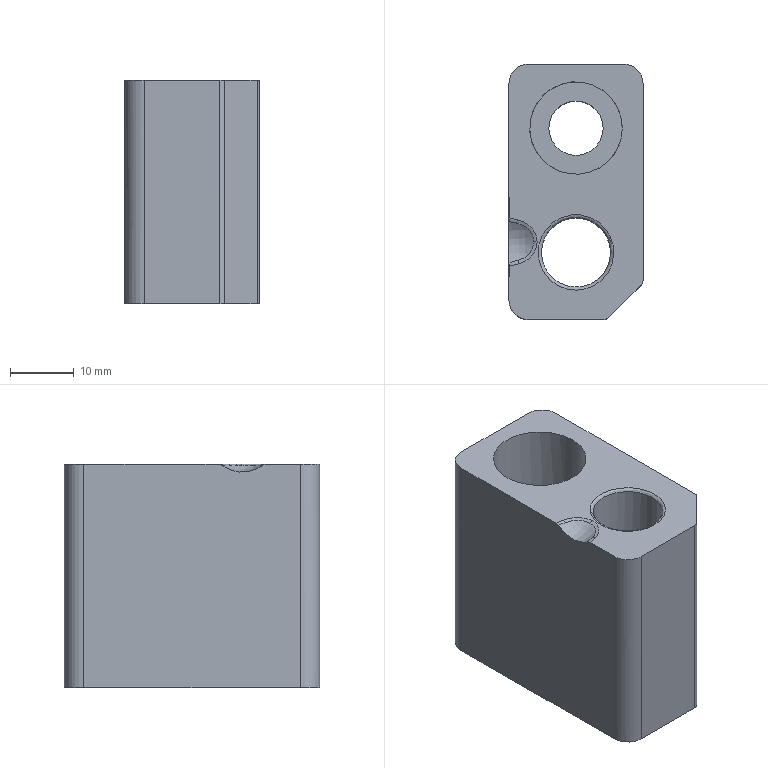Part | NX | features DIE-21 2 | 1 solid | 24 faces | box 21.001 x 40 x 35 mm | volume 21730 mm3 | plane 9 | cylinder 9 | spline 5 | torus 1 | commonest cylinder face diameters 6 x3 2 x2 8.506 x1 10.85 x1 14.5 x1 15 x1
STEP:
#1=CARTESIAN_POINT('',(2448.597,-804.612,858.547));
#2=VERTEX_POINT('',#1);
#3=CARTESIAN_POINT('',(2448.597,-811.041,858.549));
#4=VERTEX_POINT('',#3);
#5=CARTESIAN_POINT('',(2448.597,-804.616,858.545));
#6=CARTESIAN_POINT('',(2448.597,-805.575,857.92));
#7=CARTESIAN_POINT('',(2448.597,-807.823,857.052));
#8=CARTESIAN_POINT('',(2448.597,-810.077,857.926));
#9=CARTESIAN_POINT('',(2448.597,-811.039,858.548));
#10=B_SPLINE_CURVE_WITH_KNOTS('',3,(#5,#6,#7,#8,#9),.UNSPECIFIED.,.F.,.F.,(4,1,4),(0.0003039,0.003718,0.007132),.UNSPECIFIED.);
#11=EDGE_CURVE('',#2,#4,#10,.T.);
#12=ORIENTED_EDGE('',*,*,#11,.F.);
#13=CARTESIAN_POINT('',(2448.599,-804.048,858.716));
#14=VERTEX_POINT('',#13);
#15=CARTESIAN_POINT('',(2448.597,-804.617,858.543));
#16=CARTESIAN_POINT('',(2448.597,-804.449,858.653));
#17=CARTESIAN_POINT('',(2448.597,-804.249,858.716));
#18=CARTESIAN_POINT('',(2448.597,-804.048,858.716));
#19=B_SPLINE_CURVE_WITH_KNOTS('',3,(#15,#16,#17,#18),.UNSPECIFIED.,.F.,.F.,(4,4),(0.,0.0006043),.UNSPECIFIED.);
#20=EDGE_CURVE('',#2,#14,#19,.T.);
#21=ORIENTED_EDGE('',*,*,#20,.T.);
#22=CARTESIAN_POINT('',(2448.597,-792.622,858.716));
#23=VERTEX_POINT('',#22);
#24=CARTESIAN_POINT('',(2448.597,-799.949,858.716));
#25=DIRECTION('',(0.,1.,0.));
#26=VECTOR('',#25,1000.);
#27=LINE('',#24,#26);
#28=EDGE_CURVE('',#14,#23,#27,.T.);
#29=ORIENTED_EDGE('',*,*,#28,.T.);
#30=CARTESIAN_POINT('',(2448.597,-782.949,858.716));
#31=VERTEX_POINT('',#30);
#32=CARTESIAN_POINT('',(2448.597,-792.622,858.716));
#33=CARTESIAN_POINT('',(2448.597,-789.398,858.716));
#34=CARTESIAN_POINT('',(2448.597,-786.173,858.716));
#35=CARTESIAN_POINT('',(2448.597,-782.949,858.716));
#36=B_SPLINE_CURVE_WITH_KNOTS('',3,(#32,#33,#34,#35),.UNSPECIFIED.,.F.,.F.,(4,4),(0.7155,1.),.UNSPECIFIED.);
#37=EDGE_CURVE('',#23,#31,#36,.T.);
#38=ORIENTED_EDGE('',*,*,#37,.T.);
#39=CARTESIAN_POINT('',(2448.597,-782.949,823.716));
#40=VERTEX_POINT('',#39);
#41=CARTESIAN_POINT('',(2448.597,-782.949,858.716));
#42=DIRECTION('',(0.,0.,-1.));
#43=VECTOR('',#42,1000.);
#44=LINE('',#41,#43);
#45=EDGE_CURVE('',#31,#40,#44,.T.);
#46=ORIENTED_EDGE('',*,*,#45,.T.);
#47=CARTESIAN_POINT('',(2448.597,-816.949,823.716));
#48=VERTEX_POINT('',#47);
#49=CARTESIAN_POINT('',(2448.597,-799.949,823.716));
#50=DIRECTION('',(0.,-1.,0.));
#51=VECTOR('',#50,1000.);
#52=LINE('',#49,#51);
#53=EDGE_CURVE('',#40,#48,#52,.T.);
#54=ORIENTED_EDGE('',*,*,#53,.T.);
#55=CARTESIAN_POINT('',(2448.597,-816.949,858.716));
#56=VERTEX_POINT('',#55);
#57=CARTESIAN_POINT('',(2448.597,-816.949,858.716));
#58=DIRECTION('',(0.,0.,-1.));
#59=VECTOR('',#58,1000.);
#60=LINE('',#57,#59);
#61=EDGE_CURVE('',#48,#56,#60,.F.);
#62=ORIENTED_EDGE('',*,*,#61,.T.);
#63=CARTESIAN_POINT('',(2448.599,-811.606,858.716));
#64=VERTEX_POINT('',#63);
#65=CARTESIAN_POINT('',(2448.597,-799.949,858.716));
#66=DIRECTION('',(0.,1.,0.));
#67=VECTOR('',#66,1000.);
#68=LINE('',#65,#67);
#69=EDGE_CURVE('',#56,#64,#68,.T.);
#70=ORIENTED_EDGE('',*,*,#69,.T.);
#71=CARTESIAN_POINT('',(2448.597,-811.042,858.55));
#72=CARTESIAN_POINT('',(2448.597,-811.21,858.658));
#73=CARTESIAN_POINT('',(2448.597,-811.407,858.716));
#74=CARTESIAN_POINT('',(2448.597,-811.607,858.716));
#75=B_SPLINE_CURVE_WITH_KNOTS('',3,(#71,#72,#73,#74),.UNSPECIFIED.,.F.,.F.,(4,4),(0.,0.0005946),.UNSPECIFIED.);
#76=EDGE_CURVE('',#4,#64,#75,.T.);
#77=ORIENTED_EDGE('',*,*,#76,.F.);
#78=EDGE_LOOP('',(#12,#21,#29,#38,#46,#54,#62,#70,#77));
#79=FACE_BOUND('',#78,.T.);
#80=CARTESIAN_POINT('',(2448.597,-799.949,858.716));
#81=DIRECTION('',(-1.,0.,0.));
#82=DIRECTION('',(0.,0.,1.));
#83=AXIS2_PLACEMENT_3D('',#80,#81,#82);
#84=PLANE('',#83);
#85=ADVANCED_FACE('',(#79),#84,.T.);
#86=CARTESIAN_POINT('',(2465.836,-792.622,858.716));
#87=VERTEX_POINT('',#86);
#88=CARTESIAN_POINT('',(2466.479,-787.763,858.716));
#89=CARTESIAN_POINT('',(2466.552,-791.853,858.716));
#90=CARTESIAN_POINT('',(2464.453,-795.106,858.716));
#91=CARTESIAN_POINT('',(2462.087,-796.76,858.716));
#92=CARTESIAN_POINT('',(2459.253,-797.386,858.716));
#93=CARTESIAN_POINT('',(2456.395,-796.879,858.716));
#94=CARTESIAN_POINT('',(2453.948,-795.318,858.716));
#95=CARTESIAN_POINT('',(2452.286,-792.938,858.716));
#96=CARTESIAN_POINT('',(2451.66,-790.104,858.716));
#97=CARTESIAN_POINT('',(2452.167,-787.246,858.716));
#98=CARTESIAN_POINT('',(2453.728,-784.8,858.716));
#99=CARTESIAN_POINT('',(2456.107,-783.137,858.716));
#100=CARTESIAN_POINT('',(2458.942,-782.512,858.716));
#101=CARTESIAN_POINT('',(2461.8,-783.018,858.716));
#102=CARTESIAN_POINT('',(2464.245,-784.58,858.716));
#103=CARTESIAN_POINT('',(2466.479,-787.763,858.716));
#104=CARTESIAN_POINT('',(2466.552,-791.853,858.716));
#105=CARTESIAN_POINT('',(2464.453,-795.106,858.716));
#106=B_SPLINE_CURVE_WITH_KNOTS('',3,(#88,#89,#90,#91,#92,#93,#94,#95,#96,#97,#98,#99,#100,#101,#102,#103,#104,#105),.UNSPECIFIED.,.T.,.F.,(1,1,1,1,1,1,1,1,1,1,1,1,1,1,1,1,1,1,1,1,1,1),(-0.1908,-0.1283,-0.06579,0.06013,0.1217,0.1842,0.2467,0.3092,0.3717,0.4342,0.4967,0.5592,0.6217,0.6842,0.7467,0.8092,0.8717,0.9342,1.06,1.122,1.184,1.247),.UNSPECIFIED.);
#107=EDGE_CURVE('',#87,#87,#106,.T.);
#108=ORIENTED_EDGE('',*,*,#107,.T.);
#109=EDGE_LOOP('',(#108));
#110=FACE_BOUND('',#109,.T.);
#111=CARTESIAN_POINT('',(2469.597,-792.622,858.716));
#112=VERTEX_POINT('',#111);
#113=CARTESIAN_POINT('',(2469.597,-813.827,858.716));
#114=VERTEX_POINT('',#113);
#115=CARTESIAN_POINT('',(2469.597,-799.949,858.716));
#116=DIRECTION('',(0.,1.,0.));
#117=VECTOR('',#116,1000.);
#118=LINE('',#115,#117);
#119=EDGE_CURVE('',#112,#114,#118,.F.);
#120=ORIENTED_EDGE('',*,*,#119,.F.);
#121=CARTESIAN_POINT('',(2469.597,-782.949,858.716));
#122=VERTEX_POINT('',#121);
#123=CARTESIAN_POINT('',(2469.597,-792.622,858.716));
#124=CARTESIAN_POINT('',(2469.597,-789.398,858.716));
#125=CARTESIAN_POINT('',(2469.597,-786.173,858.716));
#126=CARTESIAN_POINT('',(2469.597,-782.949,858.716));
#127=B_SPLINE_CURVE_WITH_KNOTS('',3,(#123,#124,#125,#126),.UNSPECIFIED.,.F.,.F.,(4,4),(0.6937,1.),.UNSPECIFIED.);
#128=EDGE_CURVE('',#122,#112,#127,.F.);
#129=ORIENTED_EDGE('',*,*,#128,.F.);
#130=CARTESIAN_POINT('',(2466.597,-779.949,858.716));
#131=VERTEX_POINT('',#130);
#132=CARTESIAN_POINT('',(2466.597,-782.949,858.716));
#133=DIRECTION('',(0.,0.,1.));
#134=DIRECTION('',(1.,0.,0.));
#135=AXIS2_PLACEMENT_3D('',#132,#133,#134);
#136=CIRCLE('',#135,3.);
#137=EDGE_CURVE('',#122,#131,#136,.T.);
#138=ORIENTED_EDGE('',*,*,#137,.T.);
#139=CARTESIAN_POINT('',(2451.597,-779.949,858.716));
#140=VERTEX_POINT('',#139);
#141=CARTESIAN_POINT('',(2459.097,-779.949,858.716));
#142=DIRECTION('',(1.,0.,0.));
#143=VECTOR('',#142,1000.);
#144=LINE('',#141,#143);
#145=EDGE_CURVE('',#140,#131,#144,.T.);
#146=ORIENTED_EDGE('',*,*,#145,.F.);
#147=CARTESIAN_POINT('',(2451.597,-782.949,858.716));
#148=DIRECTION('',(0.,0.,1.));
#149=DIRECTION('',(1.,0.,0.));
#150=AXIS2_PLACEMENT_3D('',#147,#148,#149);
#151=CIRCLE('',#150,3.);
#152=EDGE_CURVE('',#140,#31,#151,.T.);
#153=ORIENTED_EDGE('',*,*,#152,.T.);
#154=ORIENTED_EDGE('',*,*,#37,.F.);
#155=ORIENTED_EDGE('',*,*,#28,.F.);
#156=CARTESIAN_POINT('',(2449.916,-804.322,858.716));
#157=VERTEX_POINT('',#156);
#158=CARTESIAN_POINT('',(2448.605,-804.049,858.716));
#159=CARTESIAN_POINT('',(2449.038,-804.119,858.716));
#160=CARTESIAN_POINT('',(2449.482,-804.219,858.716));
#161=CARTESIAN_POINT('',(2449.916,-804.322,858.716));
#162=B_SPLINE_CURVE_WITH_KNOTS('',3,(#158,#159,#160,#161),.UNSPECIFIED.,.F.,.F.,(4,4),(0.,1.),.UNSPECIFIED.);
#163=EDGE_CURVE('',#14,#157,#162,.T.);
#164=ORIENTED_EDGE('',*,*,#163,.T.);
#165=CARTESIAN_POINT('',(2453.005,-807.702,858.716));
#166=VERTEX_POINT('',#165);
#167=CARTESIAN_POINT('',(2449.916,-804.322,858.716));
#168=CARTESIAN_POINT('',(2450.73,-804.505,858.716));
#169=CARTESIAN_POINT('',(2452.235,-805.298,858.716));
#170=CARTESIAN_POINT('',(2452.979,-806.874,858.716));
#171=CARTESIAN_POINT('',(2453.005,-807.702,858.716));
#172=B_SPLINE_CURVE_WITH_KNOTS('',3,(#167,#168,#169,#170,#171),.UNSPECIFIED.,.F.,.F.,(4,1,4),(0.,0.5,1.),.UNSPECIFIED.);
#173=EDGE_CURVE('',#157,#166,#172,.T.);
#174=ORIENTED_EDGE('',*,*,#173,.T.);
#175=CARTESIAN_POINT('',(2450.123,-811.241,858.716));
#176=VERTEX_POINT('',#175);
#177=CARTESIAN_POINT('',(2450.123,-811.241,858.716));
#178=CARTESIAN_POINT('',(2450.931,-811.042,858.716));
#179=CARTESIAN_POINT('',(2452.406,-810.173,858.716));
#180=CARTESIAN_POINT('',(2453.031,-808.516,858.716));
#181=CARTESIAN_POINT('',(2453.005,-807.702,858.716));
#182=B_SPLINE_CURVE_WITH_KNOTS('',3,(#177,#178,#179,#180,#181),.UNSPECIFIED.,.F.,.F.,(4,1,4),(0.,0.5,1.),.UNSPECIFIED.);
#183=EDGE_CURVE('',#176,#166,#182,.T.);
#184=ORIENTED_EDGE('',*,*,#183,.F.);
#185=CARTESIAN_POINT('',(2450.123,-811.241,858.716));
#186=CARTESIAN_POINT('',(2449.618,-811.366,858.716));
#187=CARTESIAN_POINT('',(2449.063,-811.507,858.716));
#188=CARTESIAN_POINT('',(2448.606,-811.605,858.716));
#189=B_SPLINE_CURVE_WITH_KNOTS('',3,(#185,#186,#187,#188),.UNSPECIFIED.,.F.,.F.,(4,4),(0.,1.),.UNSPECIFIED.);
#190=EDGE_CURVE('',#176,#64,#189,.T.);
#191=ORIENTED_EDGE('',*,*,#190,.T.);
#192=ORIENTED_EDGE('',*,*,#69,.F.);
#193=CARTESIAN_POINT('',(2451.597,-819.949,858.716));
#194=VERTEX_POINT('',#193);
#195=CARTESIAN_POINT('',(2448.597,-816.949,858.716));
#196=CARTESIAN_POINT('',(2448.597,-817.744,858.716));
#197=CARTESIAN_POINT('',(2449.249,-819.294,858.716));
#198=CARTESIAN_POINT('',(2450.808,-819.949,858.716));
#199=CARTESIAN_POINT('',(2451.597,-819.949,858.716));
#200=B_SPLINE_CURVE_WITH_KNOTS('',3,(#195,#196,#197,#198,#199),.UNSPECIFIED.,.F.,.F.,(4,1,4),(0.,0.5,1.),.UNSPECIFIED.);
#201=EDGE_CURVE('',#56,#194,#200,.T.);
#202=ORIENTED_EDGE('',*,*,#201,.T.);
#203=CARTESIAN_POINT('',(2463.476,-819.949,858.716));
#204=VERTEX_POINT('',#203);
#205=CARTESIAN_POINT('',(2459.097,-819.949,858.716));
#206=DIRECTION('',(1.,0.,0.));
#207=VECTOR('',#206,1000.);
#208=LINE('',#205,#207);
#209=EDGE_CURVE('',#204,#194,#208,.F.);
#210=ORIENTED_EDGE('',*,*,#209,.F.);
#211=CARTESIAN_POINT('',(2464.183,-819.656,858.716));
#212=VERTEX_POINT('',#211);
#213=CARTESIAN_POINT('',(2463.476,-819.949,858.716));
#214=CARTESIAN_POINT('',(2463.752,-819.949,858.716));
#215=CARTESIAN_POINT('',(2463.988,-819.851,858.716));
#216=CARTESIAN_POINT('',(2464.183,-819.656,858.716));
#217=B_SPLINE_CURVE_WITH_KNOTS('',3,(#213,#214,#215,#216),.UNSPECIFIED.,.F.,.F.,(4,4),(0.,1.),.UNSPECIFIED.);
#218=EDGE_CURVE('',#204,#212,#217,.T.);
#219=ORIENTED_EDGE('',*,*,#218,.T.);
#220=CARTESIAN_POINT('',(2469.304,-814.535,858.716));
#221=VERTEX_POINT('',#220);
#222=CARTESIAN_POINT('',(2464.183,-819.656,858.716));
#223=DIRECTION('',(0.7071,0.7071,0.));
#224=VECTOR('',#223,1000.);
#225=LINE('',#222,#224);
#226=EDGE_CURVE('',#212,#221,#225,.T.);
#227=ORIENTED_EDGE('',*,*,#226,.T.);
#228=CARTESIAN_POINT('',(2469.304,-814.535,858.716));
#229=CARTESIAN_POINT('',(2469.5,-814.339,858.716));
#230=CARTESIAN_POINT('',(2469.597,-814.104,858.716));
#231=CARTESIAN_POINT('',(2469.597,-813.827,858.716));
#232=B_SPLINE_CURVE_WITH_KNOTS('',3,(#228,#229,#230,#231),.UNSPECIFIED.,.F.,.F.,(4,4),(0.,1.),.UNSPECIFIED.);
#233=EDGE_CURVE('',#221,#114,#232,.T.);
#234=ORIENTED_EDGE('',*,*,#233,.T.);
#235=EDGE_LOOP('',(#120,#129,#138,#146,#153,#154,#155,#164,#174,#184,#191,#192,#202,#210,#219,#227,#234));
#236=FACE_BOUND('',#235,.T.);
#237=CARTESIAN_POINT('',(2453.19,-809.768,858.716));
#238=VERTEX_POINT('',#237);
#239=CARTESIAN_POINT('',(2453.572,-811.915,858.716));
#240=CARTESIAN_POINT('',(2453.203,-810.378,858.716));
#241=CARTESIAN_POINT('',(2453.171,-809.169,858.716));
#242=CARTESIAN_POINT('',(2453.257,-808.287,858.716));
#243=CARTESIAN_POINT('',(2453.596,-807.17,858.716));
#244=CARTESIAN_POINT('',(2454.146,-806.141,858.716));
#245=CARTESIAN_POINT('',(2454.887,-805.238,858.716));
#246=CARTESIAN_POINT('',(2455.789,-804.498,858.716));
#247=CARTESIAN_POINT('',(2456.819,-803.948,858.716));
#248=CARTESIAN_POINT('',(2457.936,-803.609,858.716));
#249=CARTESIAN_POINT('',(2459.097,-803.495,858.716));
#250=CARTESIAN_POINT('',(2460.259,-803.609,858.716));
#251=CARTESIAN_POINT('',(2461.376,-803.948,858.716));
#252=CARTESIAN_POINT('',(2462.405,-804.498,858.716));
#253=CARTESIAN_POINT('',(2463.307,-805.238,858.716));
#254=CARTESIAN_POINT('',(2464.048,-806.141,858.716));
#255=CARTESIAN_POINT('',(2464.598,-807.17,858.716));
#256=CARTESIAN_POINT('',(2464.937,-808.287,858.716));
#257=CARTESIAN_POINT('',(2465.051,-809.449,858.716));
#258=CARTESIAN_POINT('',(2464.937,-810.61,858.716));
#259=CARTESIAN_POINT('',(2464.598,-811.727,858.716));
#260=CARTESIAN_POINT('',(2464.048,-812.757,858.716));
#261=CARTESIAN_POINT('',(2463.307,-813.659,858.716));
#262=CARTESIAN_POINT('',(2462.405,-814.399,858.716));
#263=CARTESIAN_POINT('',(2461.376,-814.95,858.716));
#264=CARTESIAN_POINT('',(2460.259,-815.289,858.716));
#265=CARTESIAN_POINT('',(2459.097,-815.403,858.716));
#266=CARTESIAN_POINT('',(2457.936,-815.289,858.716));
#267=CARTESIAN_POINT('',(2456.819,-814.95,858.716));
#268=CARTESIAN_POINT('',(2455.789,-814.399,858.716));
#269=CARTESIAN_POINT('',(2454.63,-813.449,858.716));
#270=CARTESIAN_POINT('',(2453.572,-811.915,858.716));
#271=CARTESIAN_POINT('',(2453.203,-810.378,858.716));
#272=CARTESIAN_POINT('',(2453.171,-809.169,858.716));
#273=B_SPLINE_CURVE_WITH_KNOTS('',3,(#239,#240,#241,#242,#243,#244,#245,#246,#247,#248,#249,#250,#251,#252,#253,#254,#255,#256,#257,#258,#259,#260,#261,#262,#263,#264,#265,#266,#267,#268,#269,#270,#271,#272),.UNSPECIFIED.,.T.,.F.,(1,1,1,1,1,1,1,1,1,1,1,1,1,1,1,1,1,1,1,1,1,1,1,1,1,1,1,1,1,1,1,1,1,1,1,1,1,1),(-0.1473,-0.116,-0.05801,0.,0.008607,0.03987,0.07114,0.1024,0.1337,0.1649,0.1962,0.2275,0.2587,0.29,0.3212,0.3525,0.3838,0.415,0.4463,0.4776,0.5088,0.5401,0.5714,0.6026,0.6339,0.6652,0.6964,0.7277,0.7589,0.7902,0.8215,0.8527,0.884,0.942,1.,1.009,1.04,1.071),.UNSPECIFIED.);
#274=EDGE_CURVE('',#238,#238,#273,.T.);
#275=ORIENTED_EDGE('',*,*,#274,.T.);
#276=EDGE_LOOP('',(#275));
#277=FACE_BOUND('',#276,.T.);
#278=CARTESIAN_POINT('',(2459.097,-799.949,858.716));
#279=DIRECTION('',(0.,0.,1.));
#280=DIRECTION('',(0.,-1.,0.));
#281=AXIS2_PLACEMENT_3D('',#278,#279,#280);
#282=PLANE('',#281);
#283=ADVANCED_FACE('',(#110,#236,#277),#282,.T.);
#284=CARTESIAN_POINT('',(2466.597,-809.449,823.716));
#285=VERTEX_POINT('',#284);
#286=CARTESIAN_POINT('',(2459.097,-809.449,823.716));
#287=DIRECTION('',(0.,0.,1.));
#288=DIRECTION('',(1.,0.,0.));
#289=AXIS2_PLACEMENT_3D('',#286,#287,#288);
#290=CIRCLE('',#289,7.5);
#291=EDGE_CURVE('',#285,#285,#290,.T.);
#292=ORIENTED_EDGE('',*,*,#291,.T.);
#293=EDGE_LOOP('',(#292));
#294=FACE_BOUND('',#293,.T.);
#295=CARTESIAN_POINT('',(2454.844,-789.949,823.716));
#296=VERTEX_POINT('',#295);
#297=CARTESIAN_POINT('',(2459.097,-789.949,823.716));
#298=DIRECTION('',(0.,0.,-1.));
#299=DIRECTION('',(-1.,0.,0.));
#300=AXIS2_PLACEMENT_3D('',#297,#298,#299);
#301=CIRCLE('',#300,4.253);
#302=EDGE_CURVE('',#296,#296,#301,.T.);
#303=ORIENTED_EDGE('',*,*,#302,.F.);
#304=EDGE_LOOP('',(#303));
#305=FACE_BOUND('',#304,.T.);
#306=CARTESIAN_POINT('',(2469.597,-813.827,823.716));
#307=VERTEX_POINT('',#306);
#308=CARTESIAN_POINT('',(2469.597,-782.949,823.716));
#309=VERTEX_POINT('',#308);
#310=CARTESIAN_POINT('',(2469.597,-799.949,823.716));
#311=DIRECTION('',(0.,1.,0.));
#312=VECTOR('',#311,1000.);
#313=LINE('',#310,#312);
#314=EDGE_CURVE('',#307,#309,#313,.T.);
#315=ORIENTED_EDGE('',*,*,#314,.F.);
#316=CARTESIAN_POINT('',(2469.304,-814.535,823.716));
#317=VERTEX_POINT('',#316);
#318=CARTESIAN_POINT('',(2468.597,-813.827,823.716));
#319=DIRECTION('',(0.,0.,-1.));
#320=DIRECTION('',(-1.,0.,0.));
#321=AXIS2_PLACEMENT_3D('',#318,#319,#320);
#322=CIRCLE('',#321,1.);
#323=EDGE_CURVE('',#307,#317,#322,.T.);
#324=ORIENTED_EDGE('',*,*,#323,.T.);
#325=CARTESIAN_POINT('',(2464.183,-819.656,823.716));
#326=VERTEX_POINT('',#325);
#327=CARTESIAN_POINT('',(2471.494,-812.345,823.716));
#328=DIRECTION('',(0.7071,0.7071,0.));
#329=VECTOR('',#328,1000.);
#330=LINE('',#327,#329);
#331=EDGE_CURVE('',#317,#326,#330,.F.);
#332=ORIENTED_EDGE('',*,*,#331,.T.);
#333=CARTESIAN_POINT('',(2463.476,-819.949,823.716));
#334=VERTEX_POINT('',#333);
#335=CARTESIAN_POINT('',(2463.476,-818.949,823.716));
#336=DIRECTION('',(0.,0.,-1.));
#337=DIRECTION('',(-1.,0.,0.));
#338=AXIS2_PLACEMENT_3D('',#335,#336,#337);
#339=CIRCLE('',#338,1.);
#340=EDGE_CURVE('',#326,#334,#339,.T.);
#341=ORIENTED_EDGE('',*,*,#340,.T.);
#342=CARTESIAN_POINT('',(2451.597,-819.949,823.716));
#343=VERTEX_POINT('',#342);
#344=CARTESIAN_POINT('',(2459.097,-819.949,823.716));
#345=DIRECTION('',(1.,0.,0.));
#346=VECTOR('',#345,1000.);
#347=LINE('',#344,#346);
#348=EDGE_CURVE('',#343,#334,#347,.T.);
#349=ORIENTED_EDGE('',*,*,#348,.F.);
#350=CARTESIAN_POINT('',(2451.597,-816.949,823.716));
#351=DIRECTION('',(0.,0.,-1.));
#352=DIRECTION('',(-1.,0.,0.));
#353=AXIS2_PLACEMENT_3D('',#350,#351,#352);
#354=CIRCLE('',#353,3.);
#355=EDGE_CURVE('',#343,#48,#354,.T.);
#356=ORIENTED_EDGE('',*,*,#355,.T.);
#357=ORIENTED_EDGE('',*,*,#53,.F.);
#358=CARTESIAN_POINT('',(2451.597,-779.949,823.716));
#359=VERTEX_POINT('',#358);
#360=CARTESIAN_POINT('',(2451.597,-782.949,823.716));
#361=DIRECTION('',(0.,0.,-1.));
#362=DIRECTION('',(-1.,0.,0.));
#363=AXIS2_PLACEMENT_3D('',#360,#361,#362);
#364=CIRCLE('',#363,3.);
#365=EDGE_CURVE('',#40,#359,#364,.T.);
#366=ORIENTED_EDGE('',*,*,#365,.T.);
#367=CARTESIAN_POINT('',(2466.597,-779.949,823.716));
#368=VERTEX_POINT('',#367);
#369=CARTESIAN_POINT('',(2459.097,-779.949,823.716));
#370=DIRECTION('',(-1.,0.,0.));
#371=VECTOR('',#370,1000.);
#372=LINE('',#369,#371);
#373=EDGE_CURVE('',#368,#359,#372,.T.);
#374=ORIENTED_EDGE('',*,*,#373,.F.);
#375=CARTESIAN_POINT('',(2466.597,-782.949,823.716));
#376=DIRECTION('',(0.,0.,-1.));
#377=DIRECTION('',(-1.,0.,0.));
#378=AXIS2_PLACEMENT_3D('',#375,#376,#377);
#379=CIRCLE('',#378,3.);
#380=EDGE_CURVE('',#368,#309,#379,.T.);
#381=ORIENTED_EDGE('',*,*,#380,.T.);
#382=EDGE_LOOP('',(#315,#324,#332,#341,#349,#356,#357,#366,#374,#381));
#383=FACE_BOUND('',#382,.T.);
#384=CARTESIAN_POINT('',(2459.097,-799.949,823.716));
#385=DIRECTION('',(0.,0.,-1.));
#386=DIRECTION('',(0.,1.,0.));
#387=AXIS2_PLACEMENT_3D('',#384,#385,#386);
#388=PLANE('',#387);
#389=ADVANCED_FACE('',(#294,#305,#383),#388,.T.);
#390=ORIENTED_EDGE('',*,*,#348,.T.);
#391=CARTESIAN_POINT('',(2463.476,-819.949,858.716));
#392=DIRECTION('',(0.,0.,-1.));
#393=VECTOR('',#392,1000.);
#394=LINE('',#391,#393);
#395=EDGE_CURVE('',#334,#204,#394,.F.);
#396=ORIENTED_EDGE('',*,*,#395,.T.);
#397=ORIENTED_EDGE('',*,*,#209,.T.);
#398=CARTESIAN_POINT('',(2451.597,-819.949,858.716));
#399=DIRECTION('',(0.,0.,-1.));
#400=VECTOR('',#399,1000.);
#401=LINE('',#398,#400);
#402=EDGE_CURVE('',#194,#343,#401,.T.);
#403=ORIENTED_EDGE('',*,*,#402,.T.);
#404=EDGE_LOOP('',(#390,#396,#397,#403));
#405=FACE_BOUND('',#404,.T.);
#406=CARTESIAN_POINT('',(2459.097,-819.949,858.716));
#407=DIRECTION('',(0.,-1.,0.));
#408=DIRECTION('',(0.,0.,-1.));
#409=AXIS2_PLACEMENT_3D('',#406,#407,#408);
#410=PLANE('',#409);
#411=ADVANCED_FACE('',(#405),#410,.T.);
#412=ORIENTED_EDGE('',*,*,#128,.T.);
#413=ORIENTED_EDGE('',*,*,#119,.T.);
#414=CARTESIAN_POINT('',(2469.597,-813.827,858.716));
#415=DIRECTION('',(0.,0.,1.));
#416=VECTOR('',#415,1000.);
#417=LINE('',#414,#416);
#418=EDGE_CURVE('',#114,#307,#417,.F.);
#419=ORIENTED_EDGE('',*,*,#418,.T.);
#420=ORIENTED_EDGE('',*,*,#314,.T.);
#421=CARTESIAN_POINT('',(2469.597,-782.949,858.716));
#422=DIRECTION('',(0.,0.,-1.));
#423=VECTOR('',#422,1000.);
#424=LINE('',#421,#423);
#425=EDGE_CURVE('',#309,#122,#424,.F.);
#426=ORIENTED_EDGE('',*,*,#425,.T.);
#427=EDGE_LOOP('',(#412,#413,#419,#420,#426));
#428=FACE_BOUND('',#427,.T.);
#429=CARTESIAN_POINT('',(2469.597,-799.949,858.716));
#430=DIRECTION('',(1.,0.,0.));
#431=DIRECTION('',(0.,0.,-1.));
#432=AXIS2_PLACEMENT_3D('',#429,#430,#431);
#433=PLANE('',#432);
#434=ADVANCED_FACE('',(#428),#433,.T.);
#435=ORIENTED_EDGE('',*,*,#145,.T.);
#436=CARTESIAN_POINT('',(2466.597,-779.949,858.716));
#437=DIRECTION('',(0.,0.,-1.));
#438=VECTOR('',#437,1000.);
#439=LINE('',#436,#438);
#440=EDGE_CURVE('',#131,#368,#439,.T.);
#441=ORIENTED_EDGE('',*,*,#440,.T.);
#442=ORIENTED_EDGE('',*,*,#373,.T.);
#443=CARTESIAN_POINT('',(2451.597,-779.949,858.716));
#444=DIRECTION('',(0.,0.,-1.));
#445=VECTOR('',#444,1000.);
#446=LINE('',#443,#445);
#447=EDGE_CURVE('',#359,#140,#446,.F.);
#448=ORIENTED_EDGE('',*,*,#447,.T.);
#449=EDGE_LOOP('',(#435,#441,#442,#448));
#450=FACE_BOUND('',#449,.T.);
#451=CARTESIAN_POINT('',(2459.097,-779.949,858.716));
#452=DIRECTION('',(0.,1.,0.));
#453=DIRECTION('',(0.,0.,1.));
#454=AXIS2_PLACEMENT_3D('',#451,#452,#453);
#455=PLANE('',#454);
#456=ADVANCED_FACE('',(#450),#455,.T.);
#457=ORIENTED_EDGE('',*,*,#331,.F.);
#458=CARTESIAN_POINT('',(2469.304,-814.535,858.716));
#459=DIRECTION('',(0.,0.,-1.));
#460=VECTOR('',#459,1000.);
#461=LINE('',#458,#460);
#462=EDGE_CURVE('',#317,#221,#461,.F.);
#463=ORIENTED_EDGE('',*,*,#462,.T.);
#464=ORIENTED_EDGE('',*,*,#226,.F.);
#465=CARTESIAN_POINT('',(2464.183,-819.656,858.716));
#466=DIRECTION('',(0.,0.,1.));
#467=VECTOR('',#466,1000.);
#468=LINE('',#465,#467);
#469=EDGE_CURVE('',#212,#326,#468,.F.);
#470=ORIENTED_EDGE('',*,*,#469,.T.);
#471=EDGE_LOOP('',(#457,#463,#464,#470));
#472=FACE_BOUND('',#471,.T.);
#473=CARTESIAN_POINT('',(2469.244,-814.595,858.716));
#474=DIRECTION('',(-0.7071,0.7071,0.));
#475=DIRECTION('',(-0.7071,-0.7071,0.));
#476=AXIS2_PLACEMENT_3D('',#473,#474,#475);
#477=PLANE('',#476);
#478=ADVANCED_FACE('',(#472),#477,.F.);
#479=ORIENTED_EDGE('',*,*,#137,.F.);
#480=ORIENTED_EDGE('',*,*,#425,.F.);
#481=ORIENTED_EDGE('',*,*,#380,.F.);
#482=ORIENTED_EDGE('',*,*,#440,.F.);
#483=EDGE_LOOP('',(#479,#480,#481,#482));
#484=FACE_BOUND('',#483,.T.);
#485=CARTESIAN_POINT('',(2466.597,-782.949,858.716));
#486=DIRECTION('',(0.,0.,-1.));
#487=DIRECTION('',(-1.,0.,0.));
#488=AXIS2_PLACEMENT_3D('',#485,#486,#487);
#489=CYLINDRICAL_SURFACE('',#488,3.);
#490=ADVANCED_FACE('',(#484),#489,.T.);
#491=ORIENTED_EDGE('',*,*,#152,.F.);
#492=ORIENTED_EDGE('',*,*,#447,.F.);
#493=ORIENTED_EDGE('',*,*,#365,.F.);
#494=ORIENTED_EDGE('',*,*,#45,.F.);
#495=EDGE_LOOP('',(#491,#492,#493,#494));
#496=FACE_BOUND('',#495,.T.);
#497=CARTESIAN_POINT('',(2451.597,-782.949,858.716));
#498=DIRECTION('',(0.,0.,-1.));
#499=DIRECTION('',(-1.,0.,0.));
#500=AXIS2_PLACEMENT_3D('',#497,#498,#499);
#501=CYLINDRICAL_SURFACE('',#500,3.);
#502=ADVANCED_FACE('',(#496),#501,.T.);
#503=ORIENTED_EDGE('',*,*,#201,.F.);
#504=ORIENTED_EDGE('',*,*,#61,.F.);
#505=ORIENTED_EDGE('',*,*,#355,.F.);
#506=ORIENTED_EDGE('',*,*,#402,.F.);
#507=EDGE_LOOP('',(#503,#504,#505,#506));
#508=FACE_BOUND('',#507,.T.);
#509=CARTESIAN_POINT('',(2451.597,-816.949,858.716));
#510=DIRECTION('',(0.,0.,-1.));
#511=DIRECTION('',(-1.,0.,0.));
#512=AXIS2_PLACEMENT_3D('',#509,#510,#511);
#513=CYLINDRICAL_SURFACE('',#512,3.);
#514=ADVANCED_FACE('',(#508),#513,.T.);
#515=ORIENTED_EDGE('',*,*,#233,.F.);
#516=ORIENTED_EDGE('',*,*,#462,.F.);
#517=ORIENTED_EDGE('',*,*,#323,.F.);
#518=ORIENTED_EDGE('',*,*,#418,.F.);
#519=EDGE_LOOP('',(#515,#516,#517,#518));
#520=FACE_BOUND('',#519,.T.);
#521=CARTESIAN_POINT('',(2468.597,-813.827,858.716));
#522=DIRECTION('',(0.,0.,1.));
#523=DIRECTION('',(1.,0.,0.));
#524=AXIS2_PLACEMENT_3D('',#521,#522,#523);
#525=CYLINDRICAL_SURFACE('',#524,1.);
#526=ADVANCED_FACE('',(#520),#525,.T.);
#527=ORIENTED_EDGE('',*,*,#340,.F.);
#528=ORIENTED_EDGE('',*,*,#469,.F.);
#529=ORIENTED_EDGE('',*,*,#218,.F.);
#530=ORIENTED_EDGE('',*,*,#395,.F.);
#531=EDGE_LOOP('',(#527,#528,#529,#530));
#532=FACE_BOUND('',#531,.T.);
#533=CARTESIAN_POINT('',(2463.476,-818.949,858.716));
#534=DIRECTION('',(0.,0.,-1.));
#535=DIRECTION('',(-1.,0.,0.));
#536=AXIS2_PLACEMENT_3D('',#533,#534,#535);
#537=CYLINDRICAL_SURFACE('',#536,1.);
#538=ADVANCED_FACE('',(#532),#537,.T.);
#539=ORIENTED_EDGE('',*,*,#302,.T.);
#540=EDGE_LOOP('',(#539));
#541=FACE_BOUND('',#540,.T.);
#542=CARTESIAN_POINT('',(2454.844,-789.949,847.716));
#543=VERTEX_POINT('',#542);
#544=CARTESIAN_POINT('',(2459.097,-789.949,847.716));
#545=DIRECTION('',(0.,0.,-1.));
#546=DIRECTION('',(-1.,0.,0.));
#547=AXIS2_PLACEMENT_3D('',#544,#545,#546);
#548=CIRCLE('',#547,4.253);
#549=EDGE_CURVE('',#543,#543,#548,.T.);
#550=ORIENTED_EDGE('',*,*,#549,.F.);
#551=EDGE_LOOP('',(#550));
#552=FACE_BOUND('',#551,.T.);
#553=CARTESIAN_POINT('',(2459.097,-789.949,858.716));
#554=DIRECTION('',(0.,0.,-1.));
#555=DIRECTION('',(1.,0.,0.));
#556=AXIS2_PLACEMENT_3D('',#553,#554,#555);
#557=CYLINDRICAL_SURFACE('',#556,4.253);
#558=ADVANCED_FACE('',(#541,#552),#557,.F.);
#559=ORIENTED_EDGE('',*,*,#549,.T.);
#560=EDGE_LOOP('',(#559));
#561=FACE_BOUND('',#560,.T.);
#562=CARTESIAN_POINT('',(2466.347,-789.949,847.716));
#563=VERTEX_POINT('',#562);
#564=CARTESIAN_POINT('',(2459.097,-789.949,847.716));
#565=DIRECTION('',(0.,0.,1.));
#566=DIRECTION('',(1.,0.,0.));
#567=AXIS2_PLACEMENT_3D('',#564,#565,#566);
#568=CIRCLE('',#567,7.25);
#569=EDGE_CURVE('',#563,#563,#568,.F.);
#570=ORIENTED_EDGE('',*,*,#569,.F.);
#571=EDGE_LOOP('',(#570));
#572=FACE_BOUND('',#571,.T.);
#573=CARTESIAN_POINT('',(2459.097,-789.949,847.716));
#574=DIRECTION('',(0.,0.,-1.));
#575=DIRECTION('',(-1.,0.,0.));
#576=AXIS2_PLACEMENT_3D('',#573,#574,#575);
#577=PLANE('',#576);
#578=ADVANCED_FACE('',(#561,#572),#577,.F.);
#579=ORIENTED_EDGE('',*,*,#569,.T.);
#580=EDGE_LOOP('',(#579));
#581=FACE_BOUND('',#580,.T.);
#582=ORIENTED_EDGE('',*,*,#107,.F.);
#583=EDGE_LOOP('',(#582));
#584=FACE_BOUND('',#583,.T.);
#585=CARTESIAN_POINT('',(2459.097,-789.949,858.716));
#586=DIRECTION('',(0.,0.,-1.));
#587=DIRECTION('',(1.,0.,0.));
#588=AXIS2_PLACEMENT_3D('',#585,#586,#587);
#589=CYLINDRICAL_SURFACE('',#588,7.25);
#590=ADVANCED_FACE('',(#581,#584),#589,.F.);
#591=ORIENTED_EDGE('',*,*,#274,.F.);
#592=EDGE_LOOP('',(#591));
#593=FACE_BOUND('',#592,.T.);
#594=CARTESIAN_POINT('',(2464.522,-809.449,858.31));
#595=VERTEX_POINT('',#594);
#596=CARTESIAN_POINT('',(2463.349,-805.2,858.31));
#597=CARTESIAN_POINT('',(2465.11,-809.447,858.31));
#598=CARTESIAN_POINT('',(2463.346,-813.705,858.31));
#599=CARTESIAN_POINT('',(2459.088,-815.461,858.31));
#600=CARTESIAN_POINT('',(2454.842,-813.694,858.31));
#601=CARTESIAN_POINT('',(2453.085,-809.447,858.31));
#602=CARTESIAN_POINT('',(2454.851,-805.192,858.31));
#603=CARTESIAN_POINT('',(2459.103,-803.438,858.31));
#604=CARTESIAN_POINT('',(2463.349,-805.2,858.31));
#605=CARTESIAN_POINT('',(2465.11,-809.447,858.31));
#606=CARTESIAN_POINT('',(2463.346,-813.705,858.31));
#607=B_SPLINE_CURVE_WITH_KNOTS('',3,(#596,#597,#598,#599,#600,#601,#602,#603,#604,#605,#606),.UNSPECIFIED.,.T.,.F.,(1,1,1,1,1,1,1,1,1,1,1,1,1,1,1),(-0.01285,-0.008565,-0.004283,0.,0.004283,0.008565,0.01285,0.01713,0.02141,0.0257,0.02998,0.03426,0.03854,0.04283,0.04711),.UNSPECIFIED.);
#608=EDGE_CURVE('',#595,#595,#607,.T.);
#609=ORIENTED_EDGE('',*,*,#608,.T.);
#610=EDGE_LOOP('',(#609));
#611=FACE_BOUND('',#610,.T.);
#612=CARTESIAN_POINT('',(2459.097,-809.449,858.216));
#613=DIRECTION('',(-0.000000005,0.,-1.));
#614=DIRECTION('',(-1.,0.,0.000000005));
#615=AXIS2_PLACEMENT_3D('',#612,#613,#614);
#616=TOROIDAL_SURFACE('',#615,5.916,0.5);
#617=ADVANCED_FACE('',(#593,#611),#616,.T.);
#618=CARTESIAN_POINT('',(2464.522,-809.449,829.216));
#619=VERTEX_POINT('',#618);
#620=CARTESIAN_POINT('',(2459.097,-809.449,829.216));
#621=DIRECTION('',(0.,0.,1.));
#622=DIRECTION('',(1.,0.,0.));
#623=AXIS2_PLACEMENT_3D('',#620,#621,#622);
#624=CIRCLE('',#623,5.425);
#625=EDGE_CURVE('',#619,#619,#624,.T.);
#626=ORIENTED_EDGE('',*,*,#625,.F.);
#627=EDGE_LOOP('',(#626));
#628=FACE_BOUND('',#627,.T.);
#629=ORIENTED_EDGE('',*,*,#608,.F.);
#630=EDGE_LOOP('',(#629));
#631=FACE_BOUND('',#630,.T.);
#632=CARTESIAN_POINT('',(2459.097,-809.449,858.3));
#633=DIRECTION('',(0.,0.,-1.));
#634=DIRECTION('',(-1.,0.,0.));
#635=AXIS2_PLACEMENT_3D('',#632,#633,#634);
#636=CYLINDRICAL_SURFACE('',#635,5.425);
#637=ADVANCED_FACE('',(#628,#631),#636,.F.);
#638=ORIENTED_EDGE('',*,*,#625,.T.);
#639=EDGE_LOOP('',(#638));
#640=FACE_BOUND('',#639,.T.);
#641=CARTESIAN_POINT('',(2466.597,-809.449,829.216));
#642=VERTEX_POINT('',#641);
#643=CARTESIAN_POINT('',(2459.097,-809.449,829.216));
#644=DIRECTION('',(0.,0.,-1.));
#645=DIRECTION('',(1.,0.,0.));
#646=AXIS2_PLACEMENT_3D('',#643,#644,#645);
#647=CIRCLE('',#646,7.5);
#648=EDGE_CURVE('',#642,#642,#647,.F.);
#649=ORIENTED_EDGE('',*,*,#648,.F.);
#650=EDGE_LOOP('',(#649));
#651=FACE_BOUND('',#650,.T.);
#652=CARTESIAN_POINT('',(2459.097,-809.449,829.216));
#653=DIRECTION('',(0.,0.,1.));
#654=DIRECTION('',(1.,0.,0.));
#655=AXIS2_PLACEMENT_3D('',#652,#653,#654);
#656=PLANE('',#655);
#657=ADVANCED_FACE('',(#640,#651),#656,.F.);
#658=ORIENTED_EDGE('',*,*,#648,.T.);
#659=EDGE_LOOP('',(#658));
#660=FACE_BOUND('',#659,.T.);
#661=ORIENTED_EDGE('',*,*,#291,.F.);
#662=EDGE_LOOP('',(#661));
#663=FACE_BOUND('',#662,.T.);
#664=CARTESIAN_POINT('',(2459.097,-809.449,823.716));
#665=DIRECTION('',(0.,0.,1.));
#666=DIRECTION('',(1.,0.,0.));
#667=AXIS2_PLACEMENT_3D('',#664,#665,#666);
#668=CYLINDRICAL_SURFACE('',#667,7.5);
#669=ADVANCED_FACE('',(#660,#663),#668,.F.);
#670=ORIENTED_EDGE('',*,*,#11,.T.);
#671=CARTESIAN_POINT('',(2449.99,-810.706,858.55));
#672=VERTEX_POINT('',#671);
#673=CARTESIAN_POINT('',(2448.597,-811.039,858.548));
#674=CARTESIAN_POINT('',(2449.079,-810.938,858.552));
#675=CARTESIAN_POINT('',(2449.469,-810.842,858.549));
#676=CARTESIAN_POINT('',(2450.005,-810.706,858.551));
#677=B_SPLINE_CURVE_WITH_KNOTS('',3,(#673,#674,#675,#676),.UNSPECIFIED.,.F.,.F.,(4,4),(0.9011,1.),.UNSPECIFIED.);
#678=EDGE_CURVE('',#672,#4,#677,.F.);
#679=ORIENTED_EDGE('',*,*,#678,.F.);
#680=CARTESIAN_POINT('',(2452.459,-807.719,858.553));
#681=VERTEX_POINT('',#680);
#682=CARTESIAN_POINT('',(2450.005,-810.706,858.551));
#683=CARTESIAN_POINT('',(2450.324,-810.626,858.553));
#684=CARTESIAN_POINT('',(2451.038,-810.35,858.541));
#685=CARTESIAN_POINT('',(2452.089,-809.484,858.567));
#686=CARTESIAN_POINT('',(2452.475,-808.378,858.55));
#687=CARTESIAN_POINT('',(2452.459,-807.719,858.553));
#688=B_SPLINE_CURVE_WITH_KNOTS('',3,(#682,#683,#684,#685,#686,#687),.UNSPECIFIED.,.F.,.F.,(4,1,1,4),(0.,0.25,0.5,1.),.UNSPECIFIED.);
#689=EDGE_CURVE('',#681,#672,#688,.F.);
#690=ORIENTED_EDGE('',*,*,#689,.F.);
#691=CARTESIAN_POINT('',(2449.811,-804.861,858.55));
#692=VERTEX_POINT('',#691);
#693=CARTESIAN_POINT('',(2452.459,-807.719,858.553));
#694=CARTESIAN_POINT('',(2452.451,-807.395,858.555));
#695=CARTESIAN_POINT('',(2452.281,-806.654,858.546));
#696=CARTESIAN_POINT('',(2451.682,-805.792,858.562));
#697=CARTESIAN_POINT('',(2450.851,-805.176,858.546));
#698=CARTESIAN_POINT('',(2450.134,-804.934,858.553));
#699=CARTESIAN_POINT('',(2449.811,-804.861,858.55));
#700=B_SPLINE_CURVE_WITH_KNOTS('',3,(#693,#694,#695,#696,#697,#698,#699),.UNSPECIFIED.,.F.,.F.,(4,1,1,1,4),(0.,0.25,0.5,0.75,1.),.UNSPECIFIED.);
#701=EDGE_CURVE('',#692,#681,#700,.F.);
#702=ORIENTED_EDGE('',*,*,#701,.F.);
#703=CARTESIAN_POINT('',(2449.811,-804.861,858.55));
#704=CARTESIAN_POINT('',(2449.388,-804.767,858.546));
#705=CARTESIAN_POINT('',(2449.024,-804.691,858.544));
#706=CARTESIAN_POINT('',(2448.596,-804.616,858.545));
#707=B_SPLINE_CURVE_WITH_KNOTS('',3,(#703,#704,#705,#706),.UNSPECIFIED.,.F.,.F.,(4,4),(0.,0.08936),.UNSPECIFIED.);
#708=EDGE_CURVE('',#2,#692,#707,.F.);
#709=ORIENTED_EDGE('',*,*,#708,.F.);
#710=EDGE_LOOP('',(#670,#679,#690,#702,#709));
#711=FACE_BOUND('',#710,.T.);
#712=CARTESIAN_POINT('',(2448.58,-811.072,858.567));
#713=CARTESIAN_POINT('',(2448.907,-811.076,858.616));
#714=CARTESIAN_POINT('',(2449.438,-811.077,858.709));
#715=CARTESIAN_POINT('',(2450.171,-811.108,858.845));
#716=CARTESIAN_POINT('',(2451.229,-811.054,859.071));
#717=CARTESIAN_POINT('',(2451.984,-810.924,859.381));
#718=CARTESIAN_POINT('',(2452.4,-810.845,859.617));
#719=CARTESIAN_POINT('',(2448.545,-810.603,858.258));
#720=CARTESIAN_POINT('',(2448.869,-810.604,858.299));
#721=CARTESIAN_POINT('',(2449.409,-810.631,858.401));
#722=CARTESIAN_POINT('',(2450.132,-810.658,858.511));
#723=CARTESIAN_POINT('',(2451.253,-810.615,858.739));
#724=CARTESIAN_POINT('',(2452.023,-810.45,859.059));
#725=CARTESIAN_POINT('',(2452.439,-810.373,859.305));
#726=CARTESIAN_POINT('',(2448.471,-809.912,857.882));
#727=CARTESIAN_POINT('',(2448.792,-809.925,857.915));
#728=CARTESIAN_POINT('',(2449.312,-809.968,857.985));
#729=CARTESIAN_POINT('',(2450.148,-809.966,858.075));
#730=CARTESIAN_POINT('',(2451.313,-809.849,858.305));
#731=CARTESIAN_POINT('',(2452.082,-809.753,858.701));
#732=CARTESIAN_POINT('',(2452.486,-809.7,858.962));
#733=CARTESIAN_POINT('',(2448.392,-808.935,857.591));
#734=CARTESIAN_POINT('',(2448.708,-808.941,857.609));
#735=CARTESIAN_POINT('',(2449.25,-808.957,857.643));
#736=CARTESIAN_POINT('',(2450.168,-808.927,857.735));
#737=CARTESIAN_POINT('',(2451.299,-808.857,858.003));
#738=CARTESIAN_POINT('',(2452.072,-808.814,858.395));
#739=CARTESIAN_POINT('',(2452.496,-808.779,858.67));
#740=CARTESIAN_POINT('',(2448.357,-808.346,857.496));
#741=CARTESIAN_POINT('',(2448.673,-808.343,857.509));
#742=CARTESIAN_POINT('',(2449.226,-808.339,857.532));
#743=CARTESIAN_POINT('',(2450.164,-808.298,857.629));
#744=CARTESIAN_POINT('',(2451.28,-808.251,857.9));
#745=CARTESIAN_POINT('',(2452.064,-808.212,858.292));
#746=CARTESIAN_POINT('',(2452.495,-808.157,858.578));
#747=CARTESIAN_POINT('',(2448.338,-807.844,857.47));
#748=CARTESIAN_POINT('',(2448.654,-807.833,857.482));
#749=CARTESIAN_POINT('',(2449.211,-807.81,857.503));
#750=CARTESIAN_POINT('',(2450.155,-807.765,857.605));
#751=CARTESIAN_POINT('',(2451.258,-807.72,857.873));
#752=CARTESIAN_POINT('',(2452.054,-807.704,858.27));
#753=CARTESIAN_POINT('',(2452.491,-807.686,858.571));
#754=CARTESIAN_POINT('',(2448.327,-807.343,857.491));
#755=CARTESIAN_POINT('',(2448.643,-807.323,857.504));
#756=CARTESIAN_POINT('',(2449.201,-807.282,857.53));
#757=CARTESIAN_POINT('',(2450.141,-807.234,857.636));
#758=CARTESIAN_POINT('',(2451.236,-807.186,857.908));
#759=CARTESIAN_POINT('',(2452.023,-807.187,858.292));
#760=CARTESIAN_POINT('',(2452.462,-807.229,858.579));
#761=CARTESIAN_POINT('',(2448.325,-806.752,857.579));
#762=CARTESIAN_POINT('',(2448.644,-806.723,857.599));
#763=CARTESIAN_POINT('',(2449.195,-806.667,857.638));
#764=CARTESIAN_POINT('',(2450.117,-806.611,857.75));
#765=CARTESIAN_POINT('',(2451.218,-806.582,858.026));
#766=CARTESIAN_POINT('',(2451.983,-806.556,858.412));
#767=CARTESIAN_POINT('',(2452.41,-806.562,858.684));
#768=CARTESIAN_POINT('',(2448.343,-805.772,857.858));
#769=CARTESIAN_POINT('',(2448.67,-805.738,857.893));
#770=CARTESIAN_POINT('',(2449.203,-805.659,857.97));
#771=CARTESIAN_POINT('',(2450.059,-805.601,858.091));
#772=CARTESIAN_POINT('',(2451.178,-805.602,858.357));
#773=CARTESIAN_POINT('',(2451.931,-805.655,858.733));
#774=CARTESIAN_POINT('',(2452.336,-805.691,858.986));
#775=CARTESIAN_POINT('',(2448.365,-805.072,858.226));
#776=CARTESIAN_POINT('',(2448.697,-805.053,858.265));
#777=CARTESIAN_POINT('',(2449.265,-804.997,858.375));
#778=CARTESIAN_POINT('',(2450.008,-804.914,858.517));
#779=CARTESIAN_POINT('',(2451.089,-804.892,858.778));
#780=CARTESIAN_POINT('',(2451.832,-804.962,859.099));
#781=CARTESIAN_POINT('',(2452.247,-805.002,859.338));
#782=CARTESIAN_POINT('',(2448.366,-804.598,858.532));
#783=CARTESIAN_POINT('',(2448.693,-804.574,858.579));
#784=CARTESIAN_POINT('',(2449.271,-804.547,858.677));
#785=CARTESIAN_POINT('',(2450.016,-804.466,858.844));
#786=CARTESIAN_POINT('',(2451.043,-804.449,859.105));
#787=CARTESIAN_POINT('',(2451.772,-804.507,859.419));
#788=CARTESIAN_POINT('',(2452.182,-804.55,859.651));
#789=B_SPLINE_SURFACE_WITH_KNOTS('',3,3,((#712,#713,#714,#715,#716,#717,#718),(#719,#720,#721,#722,#723,#724,#725),(#726,#727,#728,#729,#730,#731,#732),(#733,#734,#735,#736,#737,#738,#739),(#740,#741,#742,#743,#744,#745,#746),(#747,#748,#749,#750,#751,#752,#753),(#754,#755,#756,#757,#758,#759,#760),(#761,#762,#763,#764,#765,#766,#767),(#768,#769,#770,#771,#772,#773,#774),(#775,#776,#777,#778,#779,#780,#781),(#782,#783,#784,#785,#786,#787,#788)),.UNSPECIFIED.,.F.,.F.,.F.,(4,1,1,1,1,1,1,1,4),(4,1,1,1,4),(-0.002105,-0.001064,-0.0006303,-0.0002833,-0.00002303,0.0002372,0.0005842,0.001018,0.002059),(0.005281,0.006185,0.00683,0.007476,0.00838),.UNSPECIFIED.);
#790=ADVANCED_FACE('',(#711),#789,.F.);
#791=ORIENTED_EDGE('',*,*,#708,.T.);
#792=CARTESIAN_POINT('',(2449.916,-804.322,858.716));
#793=CARTESIAN_POINT('',(2449.874,-804.509,858.716));
#794=CARTESIAN_POINT('',(2449.83,-804.703,858.657));
#795=CARTESIAN_POINT('',(2449.795,-804.859,858.551));
#796=B_SPLINE_CURVE_WITH_KNOTS('',3,(#792,#793,#794,#795),.UNSPECIFIED.,.F.,.F.,(4,4),(0.,0.9967),.UNSPECIFIED.);
#797=EDGE_CURVE('',#692,#157,#796,.F.);
#798=ORIENTED_EDGE('',*,*,#797,.T.);
#799=ORIENTED_EDGE('',*,*,#163,.F.);
#800=ORIENTED_EDGE('',*,*,#20,.F.);
#801=EDGE_LOOP('',(#791,#798,#799,#800));
#802=FACE_BOUND('',#801,.T.);
#803=CARTESIAN_POINT('',(2448.589,-804.046,858.716));
#804=CARTESIAN_POINT('',(2449.036,-804.115,858.716));
#805=CARTESIAN_POINT('',(2449.475,-804.222,858.716));
#806=CARTESIAN_POINT('',(2449.916,-804.322,858.716));
#807=CARTESIAN_POINT('',(2448.552,-804.242,858.717));
#808=CARTESIAN_POINT('',(2449.,-804.311,858.717));
#809=CARTESIAN_POINT('',(2449.434,-804.417,858.717));
#810=CARTESIAN_POINT('',(2449.872,-804.516,858.717));
#811=CARTESIAN_POINT('',(2448.517,-804.428,858.658));
#812=CARTESIAN_POINT('',(2448.965,-804.497,858.658));
#813=CARTESIAN_POINT('',(2449.394,-804.601,858.658));
#814=CARTESIAN_POINT('',(2449.831,-804.7,858.658));
#815=CARTESIAN_POINT('',(2448.484,-804.603,858.54));
#816=CARTESIAN_POINT('',(2448.933,-804.673,858.54));
#817=CARTESIAN_POINT('',(2449.356,-804.776,858.54));
#818=CARTESIAN_POINT('',(2449.792,-804.874,858.54));
#819=B_SPLINE_SURFACE_WITH_KNOTS('',3,3,((#803,#804,#805,#806),(#807,#808,#809,#810),(#811,#812,#813,#814),(#815,#816,#817,#818)),.UNSPECIFIED.,.F.,.F.,.F.,(4,4),(4,4),(0.,1.01),(0.9089,1.),.UNSPECIFIED.);
#820=ADVANCED_FACE('',(#802),#819,.T.);
#821=ORIENTED_EDGE('',*,*,#797,.F.);
#822=ORIENTED_EDGE('',*,*,#701,.T.);
#823=CARTESIAN_POINT('',(2453.005,-807.702,858.716));
#824=CARTESIAN_POINT('',(2452.815,-807.708,858.716));
#825=CARTESIAN_POINT('',(2452.618,-807.714,858.658));
#826=CARTESIAN_POINT('',(2452.459,-807.719,858.554));
#827=B_SPLINE_CURVE_WITH_KNOTS('',3,(#823,#824,#825,#826),.UNSPECIFIED.,.F.,.F.,(4,4),(0.,0.9879),.UNSPECIFIED.);
#828=EDGE_CURVE('',#681,#166,#827,.F.);
#829=ORIENTED_EDGE('',*,*,#828,.T.);
#830=ORIENTED_EDGE('',*,*,#173,.F.);
#831=EDGE_LOOP('',(#821,#822,#829,#830));
#832=FACE_BOUND('',#831,.T.);
#833=CARTESIAN_POINT('',(2449.916,-804.322,858.716));
#834=CARTESIAN_POINT('',(2450.384,-804.427,858.716));
#835=CARTESIAN_POINT('',(2451.16,-804.736,858.716));
#836=CARTESIAN_POINT('',(2452.077,-805.461,858.716));
#837=CARTESIAN_POINT('',(2452.774,-806.41,858.716));
#838=CARTESIAN_POINT('',(2452.99,-807.223,858.716));
#839=CARTESIAN_POINT('',(2453.005,-807.702,858.716));
#840=CARTESIAN_POINT('',(2449.874,-804.509,858.717));
#841=CARTESIAN_POINT('',(2450.337,-804.613,858.717));
#842=CARTESIAN_POINT('',(2451.077,-804.894,858.717));
#843=CARTESIAN_POINT('',(2451.932,-805.577,858.717));
#844=CARTESIAN_POINT('',(2452.598,-806.489,858.717));
#845=CARTESIAN_POINT('',(2452.802,-807.238,858.717));
#846=CARTESIAN_POINT('',(2452.813,-807.708,858.717));
#847=CARTESIAN_POINT('',(2449.83,-804.704,858.657));
#848=CARTESIAN_POINT('',(2450.279,-804.804,858.657));
#849=CARTESIAN_POINT('',(2450.989,-805.057,858.663));
#850=CARTESIAN_POINT('',(2451.784,-805.703,858.66));
#851=CARTESIAN_POINT('',(2452.411,-806.561,858.658));
#852=CARTESIAN_POINT('',(2452.608,-807.259,858.659));
#853=CARTESIAN_POINT('',(2452.613,-807.715,858.657));
#854=CARTESIAN_POINT('',(2449.795,-804.86,858.55));
#855=CARTESIAN_POINT('',(2450.213,-804.954,858.55));
#856=CARTESIAN_POINT('',(2450.9,-805.175,858.56));
#857=CARTESIAN_POINT('',(2451.68,-805.829,858.554));
#858=CARTESIAN_POINT('',(2452.232,-806.56,858.553));
#859=CARTESIAN_POINT('',(2452.462,-807.306,858.553));
#860=CARTESIAN_POINT('',(2452.453,-807.72,858.55));
#861=B_SPLINE_SURFACE_WITH_KNOTS('',3,3,((#833,#834,#835,#836,#837,#838,#839),(#840,#841,#842,#843,#844,#845,#846),(#847,#848,#849,#850,#851,#852,#853),(#854,#855,#856,#857,#858,#859,#860)),.UNSPECIFIED.,.F.,.F.,.F.,(4,4),(4,1,1,1,4),(0.,1.),(0.,0.2917,0.5,0.7083,1.),.UNSPECIFIED.);
#862=ADVANCED_FACE('',(#832),#861,.T.);
#863=ORIENTED_EDGE('',*,*,#828,.F.);
#864=ORIENTED_EDGE('',*,*,#689,.T.);
#865=CARTESIAN_POINT('',(2450.123,-811.241,858.716));
#866=CARTESIAN_POINT('',(2450.077,-811.055,858.716));
#867=CARTESIAN_POINT('',(2450.029,-810.861,858.656));
#868=CARTESIAN_POINT('',(2449.99,-810.706,858.55));
#869=B_SPLINE_CURVE_WITH_KNOTS('',3,(#865,#866,#867,#868),.UNSPECIFIED.,.F.,.F.,(4,4),(0.,0.9996),.UNSPECIFIED.);
#870=EDGE_CURVE('',#176,#672,#869,.T.);
#871=ORIENTED_EDGE('',*,*,#870,.F.);
#872=ORIENTED_EDGE('',*,*,#183,.T.);
#873=EDGE_LOOP('',(#863,#864,#871,#872));
#874=FACE_BOUND('',#873,.T.);
#875=CARTESIAN_POINT('',(2453.005,-807.702,858.716));
#876=CARTESIAN_POINT('',(2453.02,-808.182,858.716));
#877=CARTESIAN_POINT('',(2452.851,-809.003,858.716));
#878=CARTESIAN_POINT('',(2452.232,-810.007,858.716));
#879=CARTESIAN_POINT('',(2451.356,-810.787,858.716));
#880=CARTESIAN_POINT('',(2450.589,-811.126,858.716));
#881=CARTESIAN_POINT('',(2450.123,-811.241,858.716));
#882=CARTESIAN_POINT('',(2452.813,-807.708,858.717));
#883=CARTESIAN_POINT('',(2452.83,-808.18,858.717));
#884=CARTESIAN_POINT('',(2452.671,-808.934,858.717));
#885=CARTESIAN_POINT('',(2452.082,-809.897,858.717));
#886=CARTESIAN_POINT('',(2451.268,-810.635,858.717));
#887=CARTESIAN_POINT('',(2450.538,-810.941,858.717));
#888=CARTESIAN_POINT('',(2450.077,-811.055,858.717));
#889=CARTESIAN_POINT('',(2452.613,-807.715,858.657));
#890=CARTESIAN_POINT('',(2452.634,-808.173,858.659));
#891=CARTESIAN_POINT('',(2452.481,-808.872,858.659));
#892=CARTESIAN_POINT('',(2451.929,-809.776,858.659));
#893=CARTESIAN_POINT('',(2451.174,-810.478,858.663));
#894=CARTESIAN_POINT('',(2450.474,-810.752,858.657));
#895=CARTESIAN_POINT('',(2450.029,-810.861,858.657));
#896=CARTESIAN_POINT('',(2452.453,-807.72,858.55));
#897=CARTESIAN_POINT('',(2452.484,-808.142,858.552));
#898=CARTESIAN_POINT('',(2452.307,-808.873,858.554));
#899=CARTESIAN_POINT('',(2451.825,-809.648,858.554));
#900=CARTESIAN_POINT('',(2451.083,-810.365,858.562));
#901=CARTESIAN_POINT('',(2450.398,-810.605,858.55));
#902=CARTESIAN_POINT('',(2449.99,-810.706,858.55));
#903=B_SPLINE_SURFACE_WITH_KNOTS('',3,3,((#875,#876,#877,#878,#879,#880,#881),(#882,#883,#884,#885,#886,#887,#888),(#889,#890,#891,#892,#893,#894,#895),(#896,#897,#898,#899,#900,#901,#902)),.UNSPECIFIED.,.F.,.F.,.F.,(4,4),(4,1,1,1,4),(0.,1.),(0.,0.2917,0.5,0.7083,1.),.UNSPECIFIED.);
#904=ADVANCED_FACE('',(#874),#903,.T.);
#905=ORIENTED_EDGE('',*,*,#76,.T.);
#906=ORIENTED_EDGE('',*,*,#190,.F.);
#907=ORIENTED_EDGE('',*,*,#870,.T.);
#908=ORIENTED_EDGE('',*,*,#678,.T.);
#909=EDGE_LOOP('',(#905,#906,#907,#908));
#910=FACE_BOUND('',#909,.T.);
#911=CARTESIAN_POINT('',(2448.588,-811.609,858.716));
#912=CARTESIAN_POINT('',(2449.102,-811.499,858.716));
#913=CARTESIAN_POINT('',(2449.612,-811.368,858.716));
#914=CARTESIAN_POINT('',(2450.123,-811.241,858.716));
#915=CARTESIAN_POINT('',(2448.549,-811.413,858.715));
#916=CARTESIAN_POINT('',(2449.06,-811.303,858.715));
#917=CARTESIAN_POINT('',(2449.564,-811.173,858.715));
#918=CARTESIAN_POINT('',(2450.075,-811.047,858.715));
#919=CARTESIAN_POINT('',(2448.512,-811.232,858.66));
#920=CARTESIAN_POINT('',(2449.022,-811.123,858.66));
#921=CARTESIAN_POINT('',(2449.519,-810.995,858.66));
#922=CARTESIAN_POINT('',(2450.031,-810.869,858.66));
#923=CARTESIAN_POINT('',(2448.48,-811.068,858.55));
#924=CARTESIAN_POINT('',(2448.988,-810.959,858.55));
#925=CARTESIAN_POINT('',(2449.478,-810.832,858.55));
#926=CARTESIAN_POINT('',(2449.99,-810.706,858.55));
#927=B_SPLINE_SURFACE_WITH_KNOTS('',3,3,((#911,#912,#913,#914),(#915,#916,#917,#918),(#919,#920,#921,#922),(#923,#924,#925,#926)),.UNSPECIFIED.,.F.,.F.,.F.,(4,4),(4,4),(0.,1.),(0.8936,1.),.UNSPECIFIED.);
#928=ADVANCED_FACE('',(#910),#927,.F.);
#929=CLOSED_SHELL('',(#85,#283,#389,#411,#434,#456,#478,#490,#502,#514,#526,#538,#558,#578,#590,#617,#637,#657,#669,#790,#820,#862,#904,#928));
#930=MANIFOLD_SOLID_BREP('',#929);
#931=(LENGTH_UNIT()NAMED_UNIT(*)SI_UNIT(.MILLI.,.METRE.));
#932=UNCERTAINTY_MEASURE_WITH_UNIT(LENGTH_MEASURE(0.0508),#931,'','');
#933=(NAMED_UNIT(*)PLANE_ANGLE_UNIT()SI_UNIT($,.RADIAN.));
#934=(NAMED_UNIT(*)SI_UNIT($,.STERADIAN.)SOLID_ANGLE_UNIT());
#935=(GEOMETRIC_REPRESENTATION_CONTEXT(3)GLOBAL_UNCERTAINTY_ASSIGNED_CONTEXT((#932))GLOBAL_UNIT_ASSIGNED_CONTEXT((#931,#933,#934))REPRESENTATION_CONTEXT('',''));
#936=ADVANCED_BREP_SHAPE_REPRESENTATION('',(#930),#935);